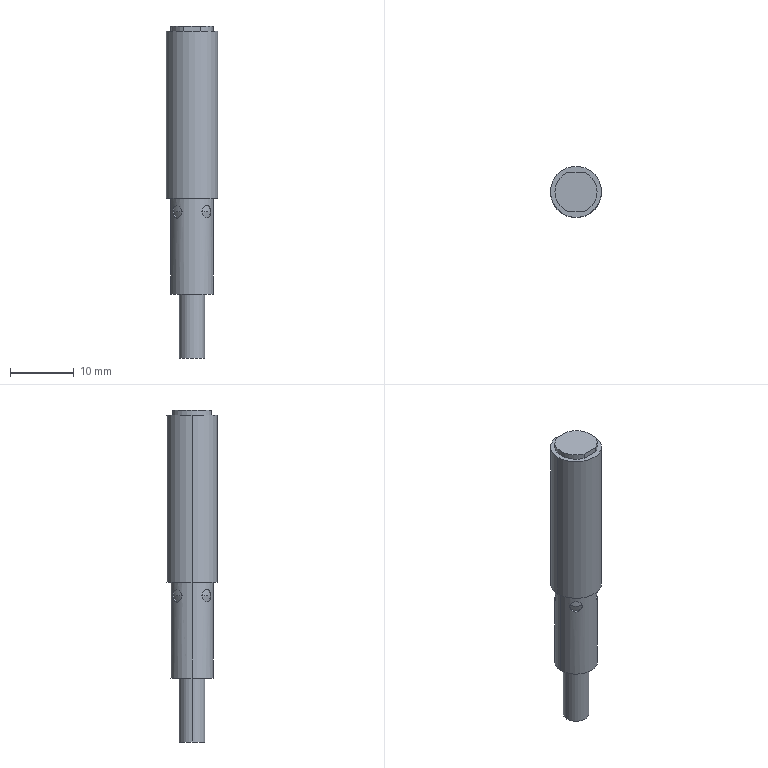Part | STEP file | E2B_S08KS01_WP_C1_BASE | 1 solid | 32 faces | box 8 x 8 x 52 mm | volume 1995 mm3 | cylinder 17 | sphere 8 | plane 7 | commonest cylinder face diameters 2 x8 6.6 x3 4 x2 6.7 x2 8 x2